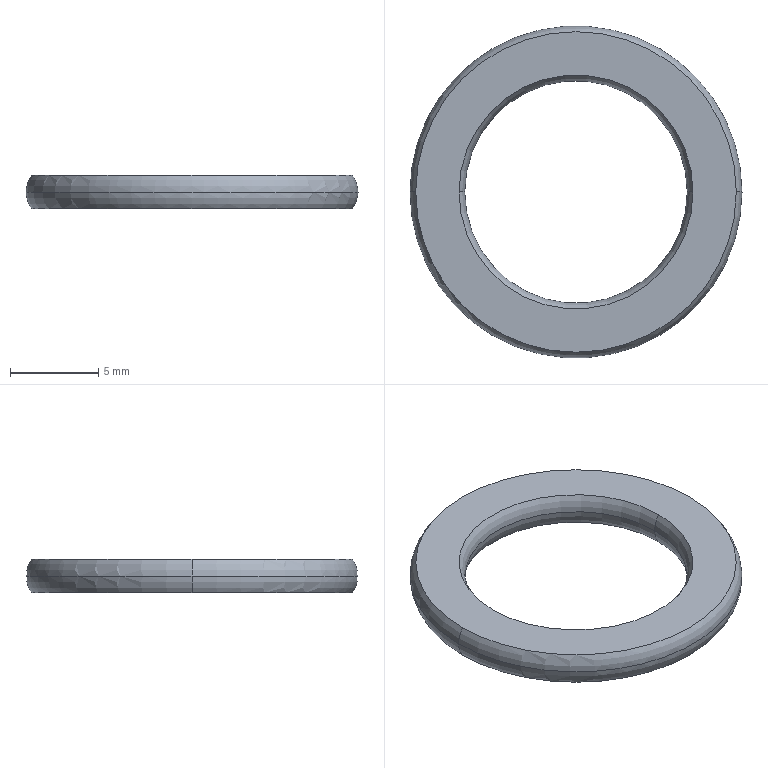Part | Creo | 1 solid | 10 faces | box 18.8 x 18.8 x 1.9 mm | volume 271.129 mm3 | torus 8 | plane 2
STEP:
#1=CARTESIAN_POINT('',(47.375,75.,105.));
#2=VERTEX_POINT('',#1);
#3=CARTESIAN_POINT('',(60.625,75.,105.));
#4=VERTEX_POINT('',#3);
#5=CARTESIAN_POINT('',(54.,75.,105.));
#6=DIRECTION('',(0.,0.,1.));
#7=DIRECTION('',(-1.,0.,0.));
#8=AXIS2_PLACEMENT_3D('',#5,#6,#7);
#9=CIRCLE('',#8,6.625);
#10=EDGE_CURVE('',#2,#4,#9,.T.);
#11=ORIENTED_EDGE('',*,*,#10,.T.);
#12=CARTESIAN_POINT('',(60.3,75.,105.95));
#13=VERTEX_POINT('',#12);
#14=CARTESIAN_POINT('',(61.85,75.,105.95));
#15=DIRECTION('',(0.,-1.,0.));
#16=DIRECTION('',(-1.,0.,0.));
#17=AXIS2_PLACEMENT_3D('',#14,#15,#16);
#18=CIRCLE('',#17,1.55);
#19=EDGE_CURVE('',#13,#4,#18,.T.);
#20=ORIENTED_EDGE('',*,*,#19,.F.);
#21=CARTESIAN_POINT('',(47.7,75.,105.95));
#22=VERTEX_POINT('',#21);
#23=CARTESIAN_POINT('',(54.,75.,105.95));
#24=DIRECTION('',(0.,0.,1.));
#25=DIRECTION('',(-1.,0.,0.));
#26=AXIS2_PLACEMENT_3D('',#23,#24,#25);
#27=CIRCLE('',#26,6.3);
#28=EDGE_CURVE('',#22,#13,#27,.T.);
#29=ORIENTED_EDGE('',*,*,#28,.F.);
#30=CARTESIAN_POINT('',(46.15,75.,105.95));
#31=DIRECTION('',(0.,1.,0.));
#32=DIRECTION('',(1.,0.,0.));
#33=AXIS2_PLACEMENT_3D('',#30,#31,#32);
#34=CIRCLE('',#33,1.55);
#35=EDGE_CURVE('',#22,#2,#34,.T.);
#36=ORIENTED_EDGE('',*,*,#35,.T.);
#37=EDGE_LOOP('',(#11,#20,#29,#36));
#38=FACE_OUTER_BOUND('',#37,.F.);
#39=CARTESIAN_POINT('',(54.,75.,105.95));
#40=DIRECTION('',(0.,0.,1.));
#41=DIRECTION('',(-1.,0.,0.));
#42=AXIS2_PLACEMENT_3D('',#39,#40,#41);
#43=TOROIDAL_SURFACE('',#42,7.85,1.55);
#44=ADVANCED_FACE('',(#38),#43,.T.);
#45=CARTESIAN_POINT('',(63.075,75.,105.));
#46=VERTEX_POINT('',#45);
#47=CARTESIAN_POINT('',(44.925,75.,105.));
#48=VERTEX_POINT('',#47);
#49=CARTESIAN_POINT('',(54.,75.,105.));
#50=DIRECTION('',(0.,0.,-1.));
#51=DIRECTION('',(1.,0.,0.));
#52=AXIS2_PLACEMENT_3D('',#49,#50,#51);
#53=CIRCLE('',#52,9.075);
#54=EDGE_CURVE('',#46,#48,#53,.T.);
#55=ORIENTED_EDGE('',*,*,#54,.F.);
#56=CARTESIAN_POINT('',(54.,75.,105.));
#57=DIRECTION('',(0.,0.,-1.));
#58=DIRECTION('',(-1.,0.,0.));
#59=AXIS2_PLACEMENT_3D('',#56,#57,#58);
#60=CIRCLE('',#59,9.075);
#61=EDGE_CURVE('',#48,#46,#60,.T.);
#62=ORIENTED_EDGE('',*,*,#61,.F.);
#63=EDGE_LOOP('',(#55,#62));
#64=FACE_OUTER_BOUND('',#63,.F.);
#65=CARTESIAN_POINT('',(54.,75.,105.));
#66=DIRECTION('',(0.,0.,1.));
#67=DIRECTION('',(1.,0.,0.));
#68=AXIS2_PLACEMENT_3D('',#65,#66,#67);
#69=CIRCLE('',#68,6.625);
#70=EDGE_CURVE('',#4,#2,#69,.T.);
#71=ORIENTED_EDGE('',*,*,#70,.F.);
#72=ORIENTED_EDGE('',*,*,#10,.F.);
#73=EDGE_LOOP('',(#71,#72));
#74=FACE_BOUND('',#73,.F.);
#75=CARTESIAN_POINT('',(54.,84.075,105.));
#76=DIRECTION('',(0.,0.,-1.));
#77=DIRECTION('',(1.,0.,0.));
#78=AXIS2_PLACEMENT_3D('',#75,#76,#77);
#79=PLANE('',#78);
#80=ADVANCED_FACE('',(#64,#74),#79,.T.);
#81=ORIENTED_EDGE('',*,*,#70,.T.);
#82=ORIENTED_EDGE('',*,*,#35,.F.);
#83=CARTESIAN_POINT('',(54.,75.,105.95));
#84=DIRECTION('',(0.,0.,1.));
#85=DIRECTION('',(1.,0.,0.));
#86=AXIS2_PLACEMENT_3D('',#83,#84,#85);
#87=CIRCLE('',#86,6.3);
#88=EDGE_CURVE('',#13,#22,#87,.T.);
#89=ORIENTED_EDGE('',*,*,#88,.F.);
#90=ORIENTED_EDGE('',*,*,#19,.T.);
#91=EDGE_LOOP('',(#81,#82,#89,#90));
#92=FACE_OUTER_BOUND('',#91,.F.);
#93=CARTESIAN_POINT('',(54.,75.,105.95));
#94=DIRECTION('',(0.,0.,1.));
#95=DIRECTION('',(-1.,0.,0.));
#96=AXIS2_PLACEMENT_3D('',#93,#94,#95);
#97=TOROIDAL_SURFACE('',#96,7.85,1.55);
#98=ADVANCED_FACE('',(#92),#97,.T.);
#99=CARTESIAN_POINT('',(47.375,75.,106.9));
#100=VERTEX_POINT('',#99);
#101=CARTESIAN_POINT('',(60.625,75.,106.9));
#102=VERTEX_POINT('',#101);
#103=CARTESIAN_POINT('',(54.,75.,106.9));
#104=DIRECTION('',(0.,0.,-1.));
#105=DIRECTION('',(-1.,0.,0.));
#106=AXIS2_PLACEMENT_3D('',#103,#104,#105);
#107=CIRCLE('',#106,6.625);
#108=EDGE_CURVE('',#100,#102,#107,.T.);
#109=ORIENTED_EDGE('',*,*,#108,.T.);
#110=CARTESIAN_POINT('',(61.85,75.,105.95));
#111=DIRECTION('',(0.,-1.,0.));
#112=DIRECTION('',(-0.7902,0.,0.6129));
#113=AXIS2_PLACEMENT_3D('',#110,#111,#112);
#114=CIRCLE('',#113,1.55);
#115=EDGE_CURVE('',#102,#13,#114,.T.);
#116=ORIENTED_EDGE('',*,*,#115,.T.);
#117=ORIENTED_EDGE('',*,*,#88,.T.);
#118=CARTESIAN_POINT('',(46.15,75.,105.95));
#119=DIRECTION('',(0.,1.,0.));
#120=DIRECTION('',(0.7902,0.,0.6129));
#121=AXIS2_PLACEMENT_3D('',#118,#119,#120);
#122=CIRCLE('',#121,1.55);
#123=EDGE_CURVE('',#100,#22,#122,.T.);
#124=ORIENTED_EDGE('',*,*,#123,.F.);
#125=EDGE_LOOP('',(#109,#116,#117,#124));
#126=FACE_OUTER_BOUND('',#125,.F.);
#127=CARTESIAN_POINT('',(54.,75.,105.95));
#128=DIRECTION('',(0.,0.,1.));
#129=DIRECTION('',(-1.,0.,0.));
#130=AXIS2_PLACEMENT_3D('',#127,#128,#129);
#131=TOROIDAL_SURFACE('',#130,7.85,1.55);
#132=ADVANCED_FACE('',(#126),#131,.T.);
#133=CARTESIAN_POINT('',(63.075,75.,106.9));
#134=VERTEX_POINT('',#133);
#135=CARTESIAN_POINT('',(44.925,75.,106.9));
#136=VERTEX_POINT('',#135);
#137=CARTESIAN_POINT('',(54.,75.,106.9));
#138=DIRECTION('',(0.,0.,1.));
#139=DIRECTION('',(1.,0.,0.));
#140=AXIS2_PLACEMENT_3D('',#137,#138,#139);
#141=CIRCLE('',#140,9.075);
#142=EDGE_CURVE('',#134,#136,#141,.T.);
#143=ORIENTED_EDGE('',*,*,#142,.F.);
#144=CARTESIAN_POINT('',(54.,75.,106.9));
#145=DIRECTION('',(0.,0.,1.));
#146=DIRECTION('',(-1.,0.,0.));
#147=AXIS2_PLACEMENT_3D('',#144,#145,#146);
#148=CIRCLE('',#147,9.075);
#149=EDGE_CURVE('',#136,#134,#148,.T.);
#150=ORIENTED_EDGE('',*,*,#149,.F.);
#151=EDGE_LOOP('',(#143,#150));
#152=FACE_OUTER_BOUND('',#151,.F.);
#153=CARTESIAN_POINT('',(54.,75.,106.9));
#154=DIRECTION('',(0.,0.,-1.));
#155=DIRECTION('',(1.,0.,0.));
#156=AXIS2_PLACEMENT_3D('',#153,#154,#155);
#157=CIRCLE('',#156,6.625);
#158=EDGE_CURVE('',#102,#100,#157,.T.);
#159=ORIENTED_EDGE('',*,*,#158,.F.);
#160=ORIENTED_EDGE('',*,*,#108,.F.);
#161=EDGE_LOOP('',(#159,#160));
#162=FACE_BOUND('',#161,.F.);
#163=CARTESIAN_POINT('',(54.,81.625,106.9));
#164=DIRECTION('',(0.,0.,1.));
#165=DIRECTION('',(-1.,0.,0.));
#166=AXIS2_PLACEMENT_3D('',#163,#164,#165);
#167=PLANE('',#166);
#168=ADVANCED_FACE('',(#152,#162),#167,.T.);
#169=ORIENTED_EDGE('',*,*,#142,.T.);
#170=CARTESIAN_POINT('',(44.6,75.,105.95));
#171=VERTEX_POINT('',#170);
#172=CARTESIAN_POINT('',(46.15,75.,105.95));
#173=DIRECTION('',(0.,1.,0.));
#174=DIRECTION('',(-1.,0.,0.));
#175=AXIS2_PLACEMENT_3D('',#172,#173,#174);
#176=CIRCLE('',#175,1.55);
#177=EDGE_CURVE('',#171,#136,#176,.T.);
#178=ORIENTED_EDGE('',*,*,#177,.F.);
#179=CARTESIAN_POINT('',(63.4,75.,105.95));
#180=VERTEX_POINT('',#179);
#181=CARTESIAN_POINT('',(54.,75.,105.95));
#182=DIRECTION('',(0.,0.,1.));
#183=DIRECTION('',(1.,0.,0.));
#184=AXIS2_PLACEMENT_3D('',#181,#182,#183);
#185=CIRCLE('',#184,9.4);
#186=EDGE_CURVE('',#180,#171,#185,.T.);
#187=ORIENTED_EDGE('',*,*,#186,.F.);
#188=CARTESIAN_POINT('',(61.85,75.,105.95));
#189=DIRECTION('',(0.,-1.,0.));
#190=DIRECTION('',(1.,0.,0.));
#191=AXIS2_PLACEMENT_3D('',#188,#189,#190);
#192=CIRCLE('',#191,1.55);
#193=EDGE_CURVE('',#180,#134,#192,.T.);
#194=ORIENTED_EDGE('',*,*,#193,.T.);
#195=EDGE_LOOP('',(#169,#178,#187,#194));
#196=FACE_OUTER_BOUND('',#195,.F.);
#197=CARTESIAN_POINT('',(54.,75.,105.95));
#198=DIRECTION('',(0.,0.,1.));
#199=DIRECTION('',(-1.,0.,0.));
#200=AXIS2_PLACEMENT_3D('',#197,#198,#199);
#201=TOROIDAL_SURFACE('',#200,7.85,1.55);
#202=ADVANCED_FACE('',(#196),#201,.T.);
#203=ORIENTED_EDGE('',*,*,#149,.T.);
#204=ORIENTED_EDGE('',*,*,#193,.F.);
#205=CARTESIAN_POINT('',(54.,75.,105.95));
#206=DIRECTION('',(0.,0.,1.));
#207=DIRECTION('',(-1.,0.,0.));
#208=AXIS2_PLACEMENT_3D('',#205,#206,#207);
#209=CIRCLE('',#208,9.4);
#210=EDGE_CURVE('',#171,#180,#209,.T.);
#211=ORIENTED_EDGE('',*,*,#210,.F.);
#212=ORIENTED_EDGE('',*,*,#177,.T.);
#213=EDGE_LOOP('',(#203,#204,#211,#212));
#214=FACE_OUTER_BOUND('',#213,.F.);
#215=CARTESIAN_POINT('',(54.,75.,105.95));
#216=DIRECTION('',(0.,0.,1.));
#217=DIRECTION('',(-1.,0.,0.));
#218=AXIS2_PLACEMENT_3D('',#215,#216,#217);
#219=TOROIDAL_SURFACE('',#218,7.85,1.55);
#220=ADVANCED_FACE('',(#214),#219,.T.);
#221=ORIENTED_EDGE('',*,*,#54,.T.);
#222=CARTESIAN_POINT('',(46.15,75.,105.95));
#223=DIRECTION('',(0.,1.,0.));
#224=DIRECTION('',(-0.7902,0.,-0.6129));
#225=AXIS2_PLACEMENT_3D('',#222,#223,#224);
#226=CIRCLE('',#225,1.55);
#227=EDGE_CURVE('',#48,#171,#226,.T.);
#228=ORIENTED_EDGE('',*,*,#227,.T.);
#229=ORIENTED_EDGE('',*,*,#210,.T.);
#230=CARTESIAN_POINT('',(61.85,75.,105.95));
#231=DIRECTION('',(0.,-1.,0.));
#232=DIRECTION('',(0.7902,0.,-0.6129));
#233=AXIS2_PLACEMENT_3D('',#230,#231,#232);
#234=CIRCLE('',#233,1.55);
#235=EDGE_CURVE('',#46,#180,#234,.T.);
#236=ORIENTED_EDGE('',*,*,#235,.F.);
#237=EDGE_LOOP('',(#221,#228,#229,#236));
#238=FACE_OUTER_BOUND('',#237,.F.);
#239=CARTESIAN_POINT('',(54.,75.,105.95));
#240=DIRECTION('',(0.,0.,1.));
#241=DIRECTION('',(-1.,0.,0.));
#242=AXIS2_PLACEMENT_3D('',#239,#240,#241);
#243=TOROIDAL_SURFACE('',#242,7.85,1.55);
#244=ADVANCED_FACE('',(#238),#243,.T.);
#245=ORIENTED_EDGE('',*,*,#61,.T.);
#246=ORIENTED_EDGE('',*,*,#235,.T.);
#247=ORIENTED_EDGE('',*,*,#186,.T.);
#248=ORIENTED_EDGE('',*,*,#227,.F.);
#249=EDGE_LOOP('',(#245,#246,#247,#248));
#250=FACE_OUTER_BOUND('',#249,.F.);
#251=CARTESIAN_POINT('',(54.,75.,105.95));
#252=DIRECTION('',(0.,0.,1.));
#253=DIRECTION('',(-1.,0.,0.));
#254=AXIS2_PLACEMENT_3D('',#251,#252,#253);
#255=TOROIDAL_SURFACE('',#254,7.85,1.55);
#256=ADVANCED_FACE('',(#250),#255,.T.);
#257=ORIENTED_EDGE('',*,*,#158,.T.);
#258=ORIENTED_EDGE('',*,*,#123,.T.);
#259=ORIENTED_EDGE('',*,*,#28,.T.);
#260=ORIENTED_EDGE('',*,*,#115,.F.);
#261=EDGE_LOOP('',(#257,#258,#259,#260));
#262=FACE_OUTER_BOUND('',#261,.F.);
#263=CARTESIAN_POINT('',(54.,75.,105.95));
#264=DIRECTION('',(0.,0.,1.));
#265=DIRECTION('',(-1.,0.,0.));
#266=AXIS2_PLACEMENT_3D('',#263,#264,#265);
#267=TOROIDAL_SURFACE('',#266,7.85,1.55);
#268=ADVANCED_FACE('',(#262),#267,.T.);
#269=CLOSED_SHELL('',(#44,#80,#98,#132,#168,#202,#220,#244,#256,#268));
#270=MANIFOLD_SOLID_BREP('',#269);
#271=(LENGTH_UNIT()NAMED_UNIT(*)SI_UNIT(.MILLI.,.METRE.));
#272=UNCERTAINTY_MEASURE_WITH_UNIT(LENGTH_MEASURE(0.002665),#271,'','');
#273=(NAMED_UNIT(*)PLANE_ANGLE_UNIT()SI_UNIT($,.RADIAN.));
#274=PLANE_ANGLE_MEASURE_WITH_UNIT(PLANE_ANGLE_MEASURE(0.01745),#273);
#275=(CONVERSION_BASED_UNIT('DEGREE',#274)NAMED_UNIT(*)PLANE_ANGLE_UNIT());
#276=(NAMED_UNIT(*)SI_UNIT($,.STERADIAN.)SOLID_ANGLE_UNIT());
#277=(GEOMETRIC_REPRESENTATION_CONTEXT(3)GLOBAL_UNCERTAINTY_ASSIGNED_CONTEXT((#272))GLOBAL_UNIT_ASSIGNED_CONTEXT((#271,#275,#276))REPRESENTATION_CONTEXT('',''));
#278=ADVANCED_BREP_SHAPE_REPRESENTATION('',(#270),#277);